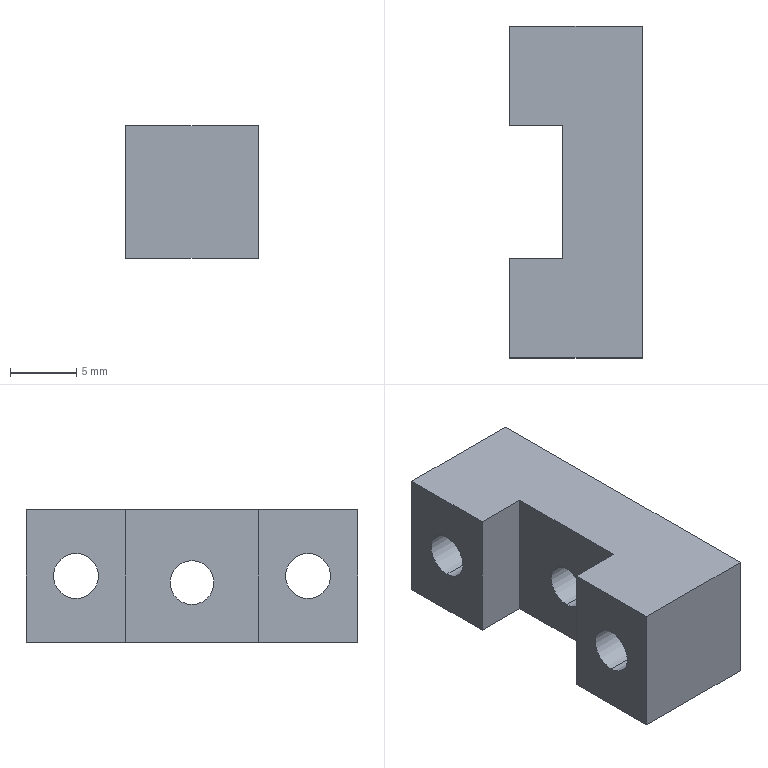Part | NX | features BREP 1 | 1 solid | 22 faces | box 10 x 25 x 10 mm | volume 1722 mm3 | plane 12 | cylinder 10 | commonest cylinder face diameters 3.4 x4 6.5 x4 3.3 x2
STEP:
#1=CARTESIAN_POINT('',(-722.471,5.279,6.15));
#2=VERTEX_POINT('',#1);
#3=CARTESIAN_POINT('',(-722.471,5.279,2.85));
#4=VERTEX_POINT('',#3);
#5=CARTESIAN_POINT('',(-722.471,5.279,4.5));
#6=DIRECTION('',(1.,0.,0.));
#7=DIRECTION('',(0.,0.,-1.));
#8=AXIS2_PLACEMENT_3D('',#5,#6,#7);
#9=CIRCLE('',#8,1.65);
#10=EDGE_CURVE('',#2,#4,#9,.T.);
#11=ORIENTED_EDGE('',*,*,#10,.F.);
#12=CARTESIAN_POINT('',(-716.471,5.279,6.15));
#13=VERTEX_POINT('',#12);
#14=CARTESIAN_POINT('',(-716.471,5.279,6.15));
#15=DIRECTION('',(1.,0.,0.));
#16=VECTOR('',#15,1000.);
#17=LINE('',#14,#16);
#18=EDGE_CURVE('',#2,#13,#17,.T.);
#19=ORIENTED_EDGE('',*,*,#18,.T.);
#20=CARTESIAN_POINT('',(-716.471,5.279,2.85));
#21=VERTEX_POINT('',#20);
#22=CARTESIAN_POINT('',(-716.471,5.279,4.5));
#23=DIRECTION('',(1.,0.,0.));
#24=DIRECTION('',(0.,0.,-1.));
#25=AXIS2_PLACEMENT_3D('',#22,#23,#24);
#26=CIRCLE('',#25,1.65);
#27=EDGE_CURVE('',#13,#21,#26,.T.);
#28=ORIENTED_EDGE('',*,*,#27,.T.);
#29=CARTESIAN_POINT('',(-716.471,5.279,2.85));
#30=DIRECTION('',(1.,0.,0.));
#31=VECTOR('',#30,1000.);
#32=LINE('',#29,#31);
#33=EDGE_CURVE('',#4,#21,#32,.T.);
#34=ORIENTED_EDGE('',*,*,#33,.F.);
#35=EDGE_LOOP('',(#11,#19,#28,#34));
#36=FACE_BOUND('',#35,.T.);
#37=CARTESIAN_POINT('',(-716.471,5.279,4.5));
#38=DIRECTION('',(1.,0.,0.));
#39=DIRECTION('',(0.,0.,-1.));
#40=AXIS2_PLACEMENT_3D('',#37,#38,#39);
#41=CYLINDRICAL_SURFACE('',#40,1.65);
#42=ADVANCED_FACE('',(#36),#41,.F.);
#43=CARTESIAN_POINT('',(-719.471,-3.471,8.25));
#44=VERTEX_POINT('',#43);
#45=CARTESIAN_POINT('',(-719.471,-3.471,1.75));
#46=VERTEX_POINT('',#45);
#47=CARTESIAN_POINT('',(-719.471,-3.471,5.));
#48=DIRECTION('',(1.,0.,0.));
#49=DIRECTION('',(0.,0.,-1.));
#50=AXIS2_PLACEMENT_3D('',#47,#48,#49);
#51=CIRCLE('',#50,3.25);
#52=EDGE_CURVE('',#44,#46,#51,.T.);
#53=ORIENTED_EDGE('',*,*,#52,.F.);
#54=CARTESIAN_POINT('',(-716.471,-3.471,8.25));
#55=VERTEX_POINT('',#54);
#56=CARTESIAN_POINT('',(-716.471,-3.471,8.25));
#57=DIRECTION('',(1.,0.,0.));
#58=VECTOR('',#57,1000.);
#59=LINE('',#56,#58);
#60=EDGE_CURVE('',#44,#55,#59,.T.);
#61=ORIENTED_EDGE('',*,*,#60,.T.);
#62=CARTESIAN_POINT('',(-716.471,-3.471,1.75));
#63=VERTEX_POINT('',#62);
#64=CARTESIAN_POINT('',(-716.471,-3.471,5.));
#65=DIRECTION('',(1.,0.,0.));
#66=DIRECTION('',(0.,0.,-1.));
#67=AXIS2_PLACEMENT_3D('',#64,#65,#66);
#68=CIRCLE('',#67,3.25);
#69=EDGE_CURVE('',#55,#63,#68,.T.);
#70=ORIENTED_EDGE('',*,*,#69,.T.);
#71=CARTESIAN_POINT('',(-716.471,-3.471,1.75));
#72=DIRECTION('',(1.,0.,0.));
#73=VECTOR('',#72,1000.);
#74=LINE('',#71,#73);
#75=EDGE_CURVE('',#46,#63,#74,.T.);
#76=ORIENTED_EDGE('',*,*,#75,.F.);
#77=EDGE_LOOP('',(#53,#61,#70,#76));
#78=FACE_BOUND('',#77,.T.);
#79=CARTESIAN_POINT('',(-716.471,-3.471,5.));
#80=DIRECTION('',(1.,0.,0.));
#81=DIRECTION('',(0.,0.,-1.));
#82=AXIS2_PLACEMENT_3D('',#79,#80,#81);
#83=CYLINDRICAL_SURFACE('',#82,3.25);
#84=ADVANCED_FACE('',(#78),#83,.F.);
#85=CARTESIAN_POINT('',(-726.471,-3.471,6.7));
#86=VERTEX_POINT('',#85);
#87=CARTESIAN_POINT('',(-726.471,-3.471,3.3));
#88=VERTEX_POINT('',#87);
#89=CARTESIAN_POINT('',(-726.471,-3.471,5.));
#90=DIRECTION('',(1.,0.,0.));
#91=DIRECTION('',(0.,0.,-1.));
#92=AXIS2_PLACEMENT_3D('',#89,#90,#91);
#93=CIRCLE('',#92,1.7);
#94=EDGE_CURVE('',#86,#88,#93,.T.);
#95=ORIENTED_EDGE('',*,*,#94,.F.);
#96=CARTESIAN_POINT('',(-719.471,-3.471,6.7));
#97=VERTEX_POINT('',#96);
#98=CARTESIAN_POINT('',(-716.471,-3.471,6.7));
#99=DIRECTION('',(1.,0.,0.));
#100=VECTOR('',#99,1000.);
#101=LINE('',#98,#100);
#102=EDGE_CURVE('',#86,#97,#101,.T.);
#103=ORIENTED_EDGE('',*,*,#102,.T.);
#104=CARTESIAN_POINT('',(-719.471,-3.471,3.3));
#105=VERTEX_POINT('',#104);
#106=CARTESIAN_POINT('',(-719.471,-3.471,5.));
#107=DIRECTION('',(1.,0.,0.));
#108=DIRECTION('',(0.,0.,-1.));
#109=AXIS2_PLACEMENT_3D('',#106,#107,#108);
#110=CIRCLE('',#109,1.7);
#111=EDGE_CURVE('',#97,#105,#110,.T.);
#112=ORIENTED_EDGE('',*,*,#111,.T.);
#113=CARTESIAN_POINT('',(-716.471,-3.471,3.3));
#114=DIRECTION('',(1.,0.,0.));
#115=VECTOR('',#114,1000.);
#116=LINE('',#113,#115);
#117=EDGE_CURVE('',#88,#105,#116,.T.);
#118=ORIENTED_EDGE('',*,*,#117,.F.);
#119=EDGE_LOOP('',(#95,#103,#112,#118));
#120=FACE_BOUND('',#119,.T.);
#121=CARTESIAN_POINT('',(-716.471,-3.471,5.));
#122=DIRECTION('',(1.,0.,0.));
#123=DIRECTION('',(0.,0.,-1.));
#124=AXIS2_PLACEMENT_3D('',#121,#122,#123);
#125=CYLINDRICAL_SURFACE('',#124,1.7);
#126=ADVANCED_FACE('',(#120),#125,.F.);
#127=CARTESIAN_POINT('',(-719.471,14.029,8.25));
#128=VERTEX_POINT('',#127);
#129=CARTESIAN_POINT('',(-719.471,14.029,1.75));
#130=VERTEX_POINT('',#129);
#131=CARTESIAN_POINT('',(-719.471,14.029,5.));
#132=DIRECTION('',(1.,0.,0.));
#133=DIRECTION('',(0.,0.,-1.));
#134=AXIS2_PLACEMENT_3D('',#131,#132,#133);
#135=CIRCLE('',#134,3.25);
#136=EDGE_CURVE('',#128,#130,#135,.T.);
#137=ORIENTED_EDGE('',*,*,#136,.F.);
#138=CARTESIAN_POINT('',(-716.471,14.029,8.25));
#139=VERTEX_POINT('',#138);
#140=CARTESIAN_POINT('',(-716.471,14.029,8.25));
#141=DIRECTION('',(1.,0.,0.));
#142=VECTOR('',#141,1000.);
#143=LINE('',#140,#142);
#144=EDGE_CURVE('',#128,#139,#143,.T.);
#145=ORIENTED_EDGE('',*,*,#144,.T.);
#146=CARTESIAN_POINT('',(-716.471,14.029,1.75));
#147=VERTEX_POINT('',#146);
#148=CARTESIAN_POINT('',(-716.471,14.029,5.));
#149=DIRECTION('',(1.,0.,0.));
#150=DIRECTION('',(0.,0.,-1.));
#151=AXIS2_PLACEMENT_3D('',#148,#149,#150);
#152=CIRCLE('',#151,3.25);
#153=EDGE_CURVE('',#139,#147,#152,.T.);
#154=ORIENTED_EDGE('',*,*,#153,.T.);
#155=CARTESIAN_POINT('',(-716.471,14.029,1.75));
#156=DIRECTION('',(1.,0.,0.));
#157=VECTOR('',#156,1000.);
#158=LINE('',#155,#157);
#159=EDGE_CURVE('',#130,#147,#158,.T.);
#160=ORIENTED_EDGE('',*,*,#159,.F.);
#161=EDGE_LOOP('',(#137,#145,#154,#160));
#162=FACE_BOUND('',#161,.T.);
#163=CARTESIAN_POINT('',(-716.471,14.029,5.));
#164=DIRECTION('',(1.,0.,0.));
#165=DIRECTION('',(0.,0.,-1.));
#166=AXIS2_PLACEMENT_3D('',#163,#164,#165);
#167=CYLINDRICAL_SURFACE('',#166,3.25);
#168=ADVANCED_FACE('',(#162),#167,.F.);
#169=CARTESIAN_POINT('',(-726.471,14.029,6.7));
#170=VERTEX_POINT('',#169);
#171=CARTESIAN_POINT('',(-726.471,14.029,3.3));
#172=VERTEX_POINT('',#171);
#173=CARTESIAN_POINT('',(-726.471,14.029,5.));
#174=DIRECTION('',(1.,0.,0.));
#175=DIRECTION('',(0.,0.,-1.));
#176=AXIS2_PLACEMENT_3D('',#173,#174,#175);
#177=CIRCLE('',#176,1.7);
#178=EDGE_CURVE('',#170,#172,#177,.T.);
#179=ORIENTED_EDGE('',*,*,#178,.F.);
#180=CARTESIAN_POINT('',(-719.471,14.029,6.7));
#181=VERTEX_POINT('',#180);
#182=CARTESIAN_POINT('',(-716.471,14.029,6.7));
#183=DIRECTION('',(1.,0.,0.));
#184=VECTOR('',#183,1000.);
#185=LINE('',#182,#184);
#186=EDGE_CURVE('',#170,#181,#185,.T.);
#187=ORIENTED_EDGE('',*,*,#186,.T.);
#188=CARTESIAN_POINT('',(-719.471,14.029,3.3));
#189=VERTEX_POINT('',#188);
#190=CARTESIAN_POINT('',(-719.471,14.029,5.));
#191=DIRECTION('',(1.,0.,0.));
#192=DIRECTION('',(0.,0.,-1.));
#193=AXIS2_PLACEMENT_3D('',#190,#191,#192);
#194=CIRCLE('',#193,1.7);
#195=EDGE_CURVE('',#181,#189,#194,.T.);
#196=ORIENTED_EDGE('',*,*,#195,.T.);
#197=CARTESIAN_POINT('',(-716.471,14.029,3.3));
#198=DIRECTION('',(1.,0.,0.));
#199=VECTOR('',#198,1000.);
#200=LINE('',#197,#199);
#201=EDGE_CURVE('',#172,#189,#200,.T.);
#202=ORIENTED_EDGE('',*,*,#201,.F.);
#203=EDGE_LOOP('',(#179,#187,#196,#202));
#204=FACE_BOUND('',#203,.T.);
#205=CARTESIAN_POINT('',(-716.471,14.029,5.));
#206=DIRECTION('',(1.,0.,0.));
#207=DIRECTION('',(0.,0.,-1.));
#208=AXIS2_PLACEMENT_3D('',#205,#206,#207);
#209=CYLINDRICAL_SURFACE('',#208,1.7);
#210=ADVANCED_FACE('',(#204),#209,.F.);
#211=CARTESIAN_POINT('',(-726.471,17.779,0.));
#212=VERTEX_POINT('',#211);
#213=CARTESIAN_POINT('',(-726.471,10.279,0.));
#214=VERTEX_POINT('',#213);
#215=CARTESIAN_POINT('',(-726.471,-7.221,0.));
#216=DIRECTION('',(0.,-1.,0.));
#217=VECTOR('',#216,1000.);
#218=LINE('',#215,#217);
#219=EDGE_CURVE('',#212,#214,#218,.T.);
#220=ORIENTED_EDGE('',*,*,#219,.T.);
#221=CARTESIAN_POINT('',(-726.471,10.279,10.));
#222=VERTEX_POINT('',#221);
#223=CARTESIAN_POINT('',(-726.471,10.279,0.));
#224=DIRECTION('',(0.,0.,1.));
#225=VECTOR('',#224,1000.);
#226=LINE('',#223,#225);
#227=EDGE_CURVE('',#214,#222,#226,.T.);
#228=ORIENTED_EDGE('',*,*,#227,.T.);
#229=CARTESIAN_POINT('',(-726.471,17.779,10.));
#230=VERTEX_POINT('',#229);
#231=CARTESIAN_POINT('',(-726.471,-7.221,10.));
#232=DIRECTION('',(0.,-1.,0.));
#233=VECTOR('',#232,1000.);
#234=LINE('',#231,#233);
#235=EDGE_CURVE('',#230,#222,#234,.T.);
#236=ORIENTED_EDGE('',*,*,#235,.F.);
#237=CARTESIAN_POINT('',(-726.471,17.779,10.));
#238=DIRECTION('',(0.,0.,-1.));
#239=VECTOR('',#238,1000.);
#240=LINE('',#237,#239);
#241=EDGE_CURVE('',#230,#212,#240,.T.);
#242=ORIENTED_EDGE('',*,*,#241,.T.);
#243=EDGE_LOOP('',(#220,#228,#236,#242));
#244=FACE_BOUND('',#243,.T.);
#245=CARTESIAN_POINT('',(-726.471,14.029,5.));
#246=DIRECTION('',(1.,0.,0.));
#247=DIRECTION('',(0.,0.,-1.));
#248=AXIS2_PLACEMENT_3D('',#245,#246,#247);
#249=CIRCLE('',#248,1.7);
#250=EDGE_CURVE('',#172,#170,#249,.T.);
#251=ORIENTED_EDGE('',*,*,#250,.T.);
#252=ORIENTED_EDGE('',*,*,#178,.T.);
#253=EDGE_LOOP('',(#251,#252));
#254=FACE_BOUND('',#253,.T.);
#255=CARTESIAN_POINT('',(-726.471,-7.221,10.));
#256=DIRECTION('',(1.,0.,0.));
#257=DIRECTION('',(0.,1.,0.));
#258=AXIS2_PLACEMENT_3D('',#255,#256,#257);
#259=PLANE('',#258);
#260=ADVANCED_FACE('',(#244,#254),#259,.F.);
#261=CARTESIAN_POINT('',(-716.471,-7.221,0.));
#262=VERTEX_POINT('',#261);
#263=CARTESIAN_POINT('',(-716.471,17.779,0.));
#264=VERTEX_POINT('',#263);
#265=CARTESIAN_POINT('',(-716.471,-7.221,0.));
#266=DIRECTION('',(0.,1.,0.));
#267=VECTOR('',#266,1000.);
#268=LINE('',#265,#267);
#269=EDGE_CURVE('',#262,#264,#268,.T.);
#270=ORIENTED_EDGE('',*,*,#269,.T.);
#271=CARTESIAN_POINT('',(-716.471,17.779,10.));
#272=VERTEX_POINT('',#271);
#273=CARTESIAN_POINT('',(-716.471,17.779,10.));
#274=DIRECTION('',(0.,0.,-1.));
#275=VECTOR('',#274,1000.);
#276=LINE('',#273,#275);
#277=EDGE_CURVE('',#272,#264,#276,.T.);
#278=ORIENTED_EDGE('',*,*,#277,.F.);
#279=CARTESIAN_POINT('',(-716.471,-7.221,10.));
#280=VERTEX_POINT('',#279);
#281=CARTESIAN_POINT('',(-716.471,-7.221,10.));
#282=DIRECTION('',(0.,1.,0.));
#283=VECTOR('',#282,1000.);
#284=LINE('',#281,#283);
#285=EDGE_CURVE('',#280,#272,#284,.T.);
#286=ORIENTED_EDGE('',*,*,#285,.F.);
#287=CARTESIAN_POINT('',(-716.471,-7.221,10.));
#288=DIRECTION('',(0.,0.,-1.));
#289=VECTOR('',#288,1000.);
#290=LINE('',#287,#289);
#291=EDGE_CURVE('',#280,#262,#290,.T.);
#292=ORIENTED_EDGE('',*,*,#291,.T.);
#293=EDGE_LOOP('',(#270,#278,#286,#292));
#294=FACE_BOUND('',#293,.T.);
#295=CARTESIAN_POINT('',(-716.471,5.279,4.5));
#296=DIRECTION('',(1.,0.,0.));
#297=DIRECTION('',(0.,0.,-1.));
#298=AXIS2_PLACEMENT_3D('',#295,#296,#297);
#299=CIRCLE('',#298,1.65);
#300=EDGE_CURVE('',#21,#13,#299,.T.);
#301=ORIENTED_EDGE('',*,*,#300,.F.);
#302=ORIENTED_EDGE('',*,*,#27,.F.);
#303=EDGE_LOOP('',(#301,#302));
#304=FACE_BOUND('',#303,.T.);
#305=CARTESIAN_POINT('',(-716.471,-3.471,5.));
#306=DIRECTION('',(1.,0.,0.));
#307=DIRECTION('',(0.,0.,-1.));
#308=AXIS2_PLACEMENT_3D('',#305,#306,#307);
#309=CIRCLE('',#308,3.25);
#310=EDGE_CURVE('',#63,#55,#309,.T.);
#311=ORIENTED_EDGE('',*,*,#310,.F.);
#312=ORIENTED_EDGE('',*,*,#69,.F.);
#313=EDGE_LOOP('',(#311,#312));
#314=FACE_BOUND('',#313,.T.);
#315=CARTESIAN_POINT('',(-716.471,14.029,5.));
#316=DIRECTION('',(1.,0.,0.));
#317=DIRECTION('',(0.,0.,-1.));
#318=AXIS2_PLACEMENT_3D('',#315,#316,#317);
#319=CIRCLE('',#318,3.25);
#320=EDGE_CURVE('',#147,#139,#319,.T.);
#321=ORIENTED_EDGE('',*,*,#320,.F.);
#322=ORIENTED_EDGE('',*,*,#153,.F.);
#323=EDGE_LOOP('',(#321,#322));
#324=FACE_BOUND('',#323,.T.);
#325=CARTESIAN_POINT('',(-716.471,-7.221,10.));
#326=DIRECTION('',(-1.,0.,0.));
#327=DIRECTION('',(0.,0.,1.));
#328=AXIS2_PLACEMENT_3D('',#325,#326,#327);
#329=PLANE('',#328);
#330=ADVANCED_FACE('',(#294,#304,#314,#324),#329,.F.);
#331=CARTESIAN_POINT('',(-716.471,17.779,0.));
#332=DIRECTION('',(-1.,0.,0.));
#333=VECTOR('',#332,1000.);
#334=LINE('',#331,#333);
#335=EDGE_CURVE('',#264,#212,#334,.T.);
#336=ORIENTED_EDGE('',*,*,#335,.T.);
#337=ORIENTED_EDGE('',*,*,#241,.F.);
#338=CARTESIAN_POINT('',(-716.471,17.779,10.));
#339=DIRECTION('',(-1.,0.,0.));
#340=VECTOR('',#339,1000.);
#341=LINE('',#338,#340);
#342=EDGE_CURVE('',#272,#230,#341,.T.);
#343=ORIENTED_EDGE('',*,*,#342,.F.);
#344=ORIENTED_EDGE('',*,*,#277,.T.);
#345=EDGE_LOOP('',(#336,#337,#343,#344));
#346=FACE_BOUND('',#345,.T.);
#347=CARTESIAN_POINT('',(-716.471,17.779,10.));
#348=DIRECTION('',(0.,-1.,0.));
#349=DIRECTION('',(0.,0.,-1.));
#350=AXIS2_PLACEMENT_3D('',#347,#348,#349);
#351=PLANE('',#350);
#352=ADVANCED_FACE('',(#346),#351,.F.);
#353=CARTESIAN_POINT('',(-726.471,0.279,10.));
#354=VERTEX_POINT('',#353);
#355=CARTESIAN_POINT('',(-726.471,-7.221,10.));
#356=VERTEX_POINT('',#355);
#357=CARTESIAN_POINT('',(-726.471,-7.221,10.));
#358=DIRECTION('',(0.,-1.,0.));
#359=VECTOR('',#358,1000.);
#360=LINE('',#357,#359);
#361=EDGE_CURVE('',#354,#356,#360,.T.);
#362=ORIENTED_EDGE('',*,*,#361,.F.);
#363=CARTESIAN_POINT('',(-726.471,0.279,0.));
#364=VERTEX_POINT('',#363);
#365=CARTESIAN_POINT('',(-726.471,0.279,0.));
#366=DIRECTION('',(0.,0.,1.));
#367=VECTOR('',#366,1000.);
#368=LINE('',#365,#367);
#369=EDGE_CURVE('',#364,#354,#368,.T.);
#370=ORIENTED_EDGE('',*,*,#369,.F.);
#371=CARTESIAN_POINT('',(-726.471,-7.221,0.));
#372=VERTEX_POINT('',#371);
#373=CARTESIAN_POINT('',(-726.471,-7.221,0.));
#374=DIRECTION('',(0.,-1.,0.));
#375=VECTOR('',#374,1000.);
#376=LINE('',#373,#375);
#377=EDGE_CURVE('',#364,#372,#376,.T.);
#378=ORIENTED_EDGE('',*,*,#377,.T.);
#379=CARTESIAN_POINT('',(-726.471,-7.221,10.));
#380=DIRECTION('',(0.,0.,-1.));
#381=VECTOR('',#380,1000.);
#382=LINE('',#379,#381);
#383=EDGE_CURVE('',#356,#372,#382,.T.);
#384=ORIENTED_EDGE('',*,*,#383,.F.);
#385=EDGE_LOOP('',(#362,#370,#378,#384));
#386=FACE_BOUND('',#385,.T.);
#387=CARTESIAN_POINT('',(-726.471,-3.471,5.));
#388=DIRECTION('',(1.,0.,0.));
#389=DIRECTION('',(0.,0.,-1.));
#390=AXIS2_PLACEMENT_3D('',#387,#388,#389);
#391=CIRCLE('',#390,1.7);
#392=EDGE_CURVE('',#88,#86,#391,.T.);
#393=ORIENTED_EDGE('',*,*,#392,.T.);
#394=ORIENTED_EDGE('',*,*,#94,.T.);
#395=EDGE_LOOP('',(#393,#394));
#396=FACE_BOUND('',#395,.T.);
#397=CARTESIAN_POINT('',(-726.471,-7.221,10.));
#398=DIRECTION('',(1.,0.,0.));
#399=DIRECTION('',(0.,1.,0.));
#400=AXIS2_PLACEMENT_3D('',#397,#398,#399);
#401=PLANE('',#400);
#402=ADVANCED_FACE('',(#386,#396),#401,.F.);
#403=CARTESIAN_POINT('',(-716.471,-7.221,0.));
#404=DIRECTION('',(1.,0.,0.));
#405=VECTOR('',#404,1000.);
#406=LINE('',#403,#405);
#407=EDGE_CURVE('',#372,#262,#406,.T.);
#408=ORIENTED_EDGE('',*,*,#407,.T.);
#409=ORIENTED_EDGE('',*,*,#291,.F.);
#410=CARTESIAN_POINT('',(-716.471,-7.221,10.));
#411=DIRECTION('',(1.,0.,0.));
#412=VECTOR('',#411,1000.);
#413=LINE('',#410,#412);
#414=EDGE_CURVE('',#356,#280,#413,.T.);
#415=ORIENTED_EDGE('',*,*,#414,.F.);
#416=ORIENTED_EDGE('',*,*,#383,.T.);
#417=EDGE_LOOP('',(#408,#409,#415,#416));
#418=FACE_BOUND('',#417,.T.);
#419=CARTESIAN_POINT('',(-716.471,-7.221,10.));
#420=DIRECTION('',(0.,1.,0.));
#421=DIRECTION('',(1.,0.,0.));
#422=AXIS2_PLACEMENT_3D('',#419,#420,#421);
#423=PLANE('',#422);
#424=ADVANCED_FACE('',(#418),#423,.F.);
#425=CARTESIAN_POINT('',(-722.471,10.279,10.));
#426=VERTEX_POINT('',#425);
#427=CARTESIAN_POINT('',(-726.471,10.279,10.));
#428=DIRECTION('',(-1.,0.,0.));
#429=VECTOR('',#428,1000.);
#430=LINE('',#427,#429);
#431=EDGE_CURVE('',#426,#222,#430,.T.);
#432=ORIENTED_EDGE('',*,*,#431,.F.);
#433=CARTESIAN_POINT('',(-722.471,0.279,10.));
#434=VERTEX_POINT('',#433);
#435=CARTESIAN_POINT('',(-722.471,0.279,10.));
#436=DIRECTION('',(0.,1.,0.));
#437=VECTOR('',#436,1000.);
#438=LINE('',#435,#437);
#439=EDGE_CURVE('',#434,#426,#438,.T.);
#440=ORIENTED_EDGE('',*,*,#439,.F.);
#441=CARTESIAN_POINT('',(-726.471,0.279,10.));
#442=DIRECTION('',(1.,0.,0.));
#443=VECTOR('',#442,1000.);
#444=LINE('',#441,#443);
#445=EDGE_CURVE('',#354,#434,#444,.T.);
#446=ORIENTED_EDGE('',*,*,#445,.F.);
#447=ORIENTED_EDGE('',*,*,#361,.T.);
#448=ORIENTED_EDGE('',*,*,#414,.T.);
#449=ORIENTED_EDGE('',*,*,#285,.T.);
#450=ORIENTED_EDGE('',*,*,#342,.T.);
#451=ORIENTED_EDGE('',*,*,#235,.T.);
#452=EDGE_LOOP('',(#432,#440,#446,#447,#448,#449,#450,#451));
#453=FACE_BOUND('',#452,.T.);
#454=CARTESIAN_POINT('',(-716.471,17.779,10.));
#455=DIRECTION('',(0.,0.,1.));
#456=DIRECTION('',(1.,0.,0.));
#457=AXIS2_PLACEMENT_3D('',#454,#455,#456);
#458=PLANE('',#457);
#459=ADVANCED_FACE('',(#453),#458,.T.);
#460=CARTESIAN_POINT('',(-722.471,0.279,0.));
#461=VERTEX_POINT('',#460);
#462=CARTESIAN_POINT('',(-722.471,10.279,0.));
#463=VERTEX_POINT('',#462);
#464=CARTESIAN_POINT('',(-722.471,0.279,0.));
#465=DIRECTION('',(0.,1.,0.));
#466=VECTOR('',#465,1000.);
#467=LINE('',#464,#466);
#468=EDGE_CURVE('',#461,#463,#467,.T.);
#469=ORIENTED_EDGE('',*,*,#468,.T.);
#470=CARTESIAN_POINT('',(-726.471,10.279,0.));
#471=DIRECTION('',(-1.,0.,0.));
#472=VECTOR('',#471,1000.);
#473=LINE('',#470,#472);
#474=EDGE_CURVE('',#463,#214,#473,.T.);
#475=ORIENTED_EDGE('',*,*,#474,.T.);
#476=ORIENTED_EDGE('',*,*,#219,.F.);
#477=ORIENTED_EDGE('',*,*,#335,.F.);
#478=ORIENTED_EDGE('',*,*,#269,.F.);
#479=ORIENTED_EDGE('',*,*,#407,.F.);
#480=ORIENTED_EDGE('',*,*,#377,.F.);
#481=CARTESIAN_POINT('',(-726.471,0.279,0.));
#482=DIRECTION('',(1.,0.,0.));
#483=VECTOR('',#482,1000.);
#484=LINE('',#481,#483);
#485=EDGE_CURVE('',#364,#461,#484,.T.);
#486=ORIENTED_EDGE('',*,*,#485,.T.);
#487=EDGE_LOOP('',(#469,#475,#476,#477,#478,#479,#480,#486));
#488=FACE_BOUND('',#487,.T.);
#489=CARTESIAN_POINT('',(-716.471,17.779,0.));
#490=DIRECTION('',(0.,0.,1.));
#491=DIRECTION('',(1.,0.,0.));
#492=AXIS2_PLACEMENT_3D('',#489,#490,#491);
#493=PLANE('',#492);
#494=ADVANCED_FACE('',(#488),#493,.F.);
#495=ORIENTED_EDGE('',*,*,#431,.T.);
#496=ORIENTED_EDGE('',*,*,#227,.F.);
#497=ORIENTED_EDGE('',*,*,#474,.F.);
#498=CARTESIAN_POINT('',(-722.471,10.279,0.));
#499=DIRECTION('',(0.,0.,1.));
#500=VECTOR('',#499,1000.);
#501=LINE('',#498,#500);
#502=EDGE_CURVE('',#463,#426,#501,.T.);
#503=ORIENTED_EDGE('',*,*,#502,.T.);
#504=EDGE_LOOP('',(#495,#496,#497,#503));
#505=FACE_BOUND('',#504,.T.);
#506=CARTESIAN_POINT('',(-726.471,10.279,0.));
#507=DIRECTION('',(0.,1.,0.));
#508=DIRECTION('',(1.,0.,0.));
#509=AXIS2_PLACEMENT_3D('',#506,#507,#508);
#510=PLANE('',#509);
#511=ADVANCED_FACE('',(#505),#510,.F.);
#512=ORIENTED_EDGE('',*,*,#439,.T.);
#513=ORIENTED_EDGE('',*,*,#502,.F.);
#514=ORIENTED_EDGE('',*,*,#468,.F.);
#515=CARTESIAN_POINT('',(-722.471,0.279,0.));
#516=DIRECTION('',(0.,0.,1.));
#517=VECTOR('',#516,1000.);
#518=LINE('',#515,#517);
#519=EDGE_CURVE('',#461,#434,#518,.T.);
#520=ORIENTED_EDGE('',*,*,#519,.T.);
#521=EDGE_LOOP('',(#512,#513,#514,#520));
#522=FACE_BOUND('',#521,.T.);
#523=CARTESIAN_POINT('',(-722.471,5.279,4.5));
#524=DIRECTION('',(1.,0.,0.));
#525=DIRECTION('',(0.,0.,-1.));
#526=AXIS2_PLACEMENT_3D('',#523,#524,#525);
#527=CIRCLE('',#526,1.65);
#528=EDGE_CURVE('',#4,#2,#527,.T.);
#529=ORIENTED_EDGE('',*,*,#528,.T.);
#530=ORIENTED_EDGE('',*,*,#10,.T.);
#531=EDGE_LOOP('',(#529,#530));
#532=FACE_BOUND('',#531,.T.);
#533=CARTESIAN_POINT('',(-722.471,0.279,0.));
#534=DIRECTION('',(1.,0.,0.));
#535=DIRECTION('',(0.,1.,0.));
#536=AXIS2_PLACEMENT_3D('',#533,#534,#535);
#537=PLANE('',#536);
#538=ADVANCED_FACE('',(#522,#532),#537,.F.);
#539=ORIENTED_EDGE('',*,*,#445,.T.);
#540=ORIENTED_EDGE('',*,*,#519,.F.);
#541=ORIENTED_EDGE('',*,*,#485,.F.);
#542=ORIENTED_EDGE('',*,*,#369,.T.);
#543=EDGE_LOOP('',(#539,#540,#541,#542));
#544=FACE_BOUND('',#543,.T.);
#545=CARTESIAN_POINT('',(-726.471,0.279,0.));
#546=DIRECTION('',(0.,-1.,0.));
#547=DIRECTION('',(-1.,0.,0.));
#548=AXIS2_PLACEMENT_3D('',#545,#546,#547);
#549=PLANE('',#548);
#550=ADVANCED_FACE('',(#544),#549,.F.);
#551=ORIENTED_EDGE('',*,*,#186,.F.);
#552=ORIENTED_EDGE('',*,*,#250,.F.);
#553=ORIENTED_EDGE('',*,*,#201,.T.);
#554=CARTESIAN_POINT('',(-719.471,14.029,5.));
#555=DIRECTION('',(1.,0.,0.));
#556=DIRECTION('',(0.,0.,-1.));
#557=AXIS2_PLACEMENT_3D('',#554,#555,#556);
#558=CIRCLE('',#557,1.7);
#559=EDGE_CURVE('',#189,#181,#558,.T.);
#560=ORIENTED_EDGE('',*,*,#559,.T.);
#561=EDGE_LOOP('',(#551,#552,#553,#560));
#562=FACE_BOUND('',#561,.T.);
#563=CARTESIAN_POINT('',(-716.471,14.029,5.));
#564=DIRECTION('',(1.,0.,0.));
#565=DIRECTION('',(0.,0.,-1.));
#566=AXIS2_PLACEMENT_3D('',#563,#564,#565);
#567=CYLINDRICAL_SURFACE('',#566,1.7);
#568=ADVANCED_FACE('',(#562),#567,.F.);
#569=CARTESIAN_POINT('',(-719.471,14.029,5.));
#570=DIRECTION('',(1.,0.,0.));
#571=DIRECTION('',(0.,0.,-1.));
#572=AXIS2_PLACEMENT_3D('',#569,#570,#571);
#573=CIRCLE('',#572,3.25);
#574=EDGE_CURVE('',#130,#128,#573,.T.);
#575=ORIENTED_EDGE('',*,*,#574,.T.);
#576=ORIENTED_EDGE('',*,*,#136,.T.);
#577=EDGE_LOOP('',(#575,#576));
#578=FACE_BOUND('',#577,.T.);
#579=ORIENTED_EDGE('',*,*,#559,.F.);
#580=ORIENTED_EDGE('',*,*,#195,.F.);
#581=EDGE_LOOP('',(#579,#580));
#582=FACE_BOUND('',#581,.T.);
#583=CARTESIAN_POINT('',(-719.471,15.729,5.));
#584=DIRECTION('',(-1.,0.,0.));
#585=DIRECTION('',(0.,0.,1.));
#586=AXIS2_PLACEMENT_3D('',#583,#584,#585);
#587=PLANE('',#586);
#588=ADVANCED_FACE('',(#578,#582),#587,.F.);
#589=ORIENTED_EDGE('',*,*,#144,.F.);
#590=ORIENTED_EDGE('',*,*,#574,.F.);
#591=ORIENTED_EDGE('',*,*,#159,.T.);
#592=ORIENTED_EDGE('',*,*,#320,.T.);
#593=EDGE_LOOP('',(#589,#590,#591,#592));
#594=FACE_BOUND('',#593,.T.);
#595=CARTESIAN_POINT('',(-716.471,14.029,5.));
#596=DIRECTION('',(1.,0.,0.));
#597=DIRECTION('',(0.,0.,-1.));
#598=AXIS2_PLACEMENT_3D('',#595,#596,#597);
#599=CYLINDRICAL_SURFACE('',#598,3.25);
#600=ADVANCED_FACE('',(#594),#599,.F.);
#601=ORIENTED_EDGE('',*,*,#102,.F.);
#602=ORIENTED_EDGE('',*,*,#392,.F.);
#603=ORIENTED_EDGE('',*,*,#117,.T.);
#604=CARTESIAN_POINT('',(-719.471,-3.471,5.));
#605=DIRECTION('',(1.,0.,0.));
#606=DIRECTION('',(0.,0.,-1.));
#607=AXIS2_PLACEMENT_3D('',#604,#605,#606);
#608=CIRCLE('',#607,1.7);
#609=EDGE_CURVE('',#105,#97,#608,.T.);
#610=ORIENTED_EDGE('',*,*,#609,.T.);
#611=EDGE_LOOP('',(#601,#602,#603,#610));
#612=FACE_BOUND('',#611,.T.);
#613=CARTESIAN_POINT('',(-716.471,-3.471,5.));
#614=DIRECTION('',(1.,0.,0.));
#615=DIRECTION('',(0.,0.,-1.));
#616=AXIS2_PLACEMENT_3D('',#613,#614,#615);
#617=CYLINDRICAL_SURFACE('',#616,1.7);
#618=ADVANCED_FACE('',(#612),#617,.F.);
#619=CARTESIAN_POINT('',(-719.471,-3.471,5.));
#620=DIRECTION('',(1.,0.,0.));
#621=DIRECTION('',(0.,0.,-1.));
#622=AXIS2_PLACEMENT_3D('',#619,#620,#621);
#623=CIRCLE('',#622,3.25);
#624=EDGE_CURVE('',#46,#44,#623,.T.);
#625=ORIENTED_EDGE('',*,*,#624,.T.);
#626=ORIENTED_EDGE('',*,*,#52,.T.);
#627=EDGE_LOOP('',(#625,#626));
#628=FACE_BOUND('',#627,.T.);
#629=ORIENTED_EDGE('',*,*,#609,.F.);
#630=ORIENTED_EDGE('',*,*,#111,.F.);
#631=EDGE_LOOP('',(#629,#630));
#632=FACE_BOUND('',#631,.T.);
#633=CARTESIAN_POINT('',(-719.471,-1.771,5.));
#634=DIRECTION('',(-1.,0.,0.));
#635=DIRECTION('',(0.,0.,1.));
#636=AXIS2_PLACEMENT_3D('',#633,#634,#635);
#637=PLANE('',#636);
#638=ADVANCED_FACE('',(#628,#632),#637,.F.);
#639=ORIENTED_EDGE('',*,*,#60,.F.);
#640=ORIENTED_EDGE('',*,*,#624,.F.);
#641=ORIENTED_EDGE('',*,*,#75,.T.);
#642=ORIENTED_EDGE('',*,*,#310,.T.);
#643=EDGE_LOOP('',(#639,#640,#641,#642));
#644=FACE_BOUND('',#643,.T.);
#645=CARTESIAN_POINT('',(-716.471,-3.471,5.));
#646=DIRECTION('',(1.,0.,0.));
#647=DIRECTION('',(0.,0.,-1.));
#648=AXIS2_PLACEMENT_3D('',#645,#646,#647);
#649=CYLINDRICAL_SURFACE('',#648,3.25);
#650=ADVANCED_FACE('',(#644),#649,.F.);
#651=ORIENTED_EDGE('',*,*,#18,.F.);
#652=ORIENTED_EDGE('',*,*,#528,.F.);
#653=ORIENTED_EDGE('',*,*,#33,.T.);
#654=ORIENTED_EDGE('',*,*,#300,.T.);
#655=EDGE_LOOP('',(#651,#652,#653,#654));
#656=FACE_BOUND('',#655,.T.);
#657=CARTESIAN_POINT('',(-716.471,5.279,4.5));
#658=DIRECTION('',(1.,0.,0.));
#659=DIRECTION('',(0.,0.,-1.));
#660=AXIS2_PLACEMENT_3D('',#657,#658,#659);
#661=CYLINDRICAL_SURFACE('',#660,1.65);
#662=ADVANCED_FACE('',(#656),#661,.F.);
#663=CLOSED_SHELL('',(#42,#84,#126,#168,#210,#260,#330,#352,#402,#424,#459,#494,#511,#538,#550,#568,#588,#600,#618,#638,#650,#662));
#664=MANIFOLD_SOLID_BREP('',#663);
#665=(LENGTH_UNIT()NAMED_UNIT(*)SI_UNIT(.MILLI.,.METRE.));
#666=UNCERTAINTY_MEASURE_WITH_UNIT(LENGTH_MEASURE(0.00001),#665,'','');
#667=(NAMED_UNIT(*)PLANE_ANGLE_UNIT()SI_UNIT($,.RADIAN.));
#668=(NAMED_UNIT(*)SI_UNIT($,.STERADIAN.)SOLID_ANGLE_UNIT());
#669=(GEOMETRIC_REPRESENTATION_CONTEXT(3)GLOBAL_UNCERTAINTY_ASSIGNED_CONTEXT((#666))GLOBAL_UNIT_ASSIGNED_CONTEXT((#665,#667,#668))REPRESENTATION_CONTEXT('',''));
#670=ADVANCED_BREP_SHAPE_REPRESENTATION('',(#664),#669);